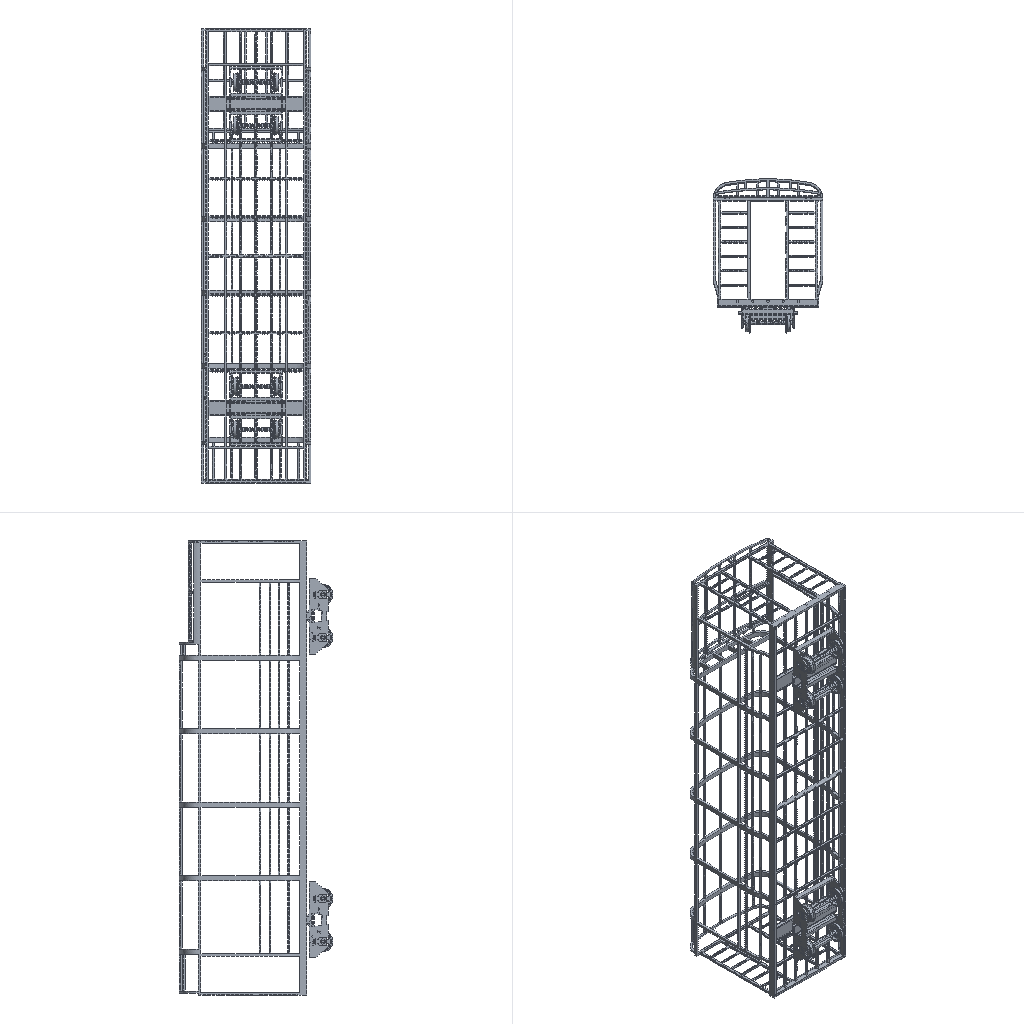Simulation study | ansys workbench
Set-up summary:
category,name,step,type,value,unit,region
solver,ansys_workbench
units,mm-N-s-tonne (MPa),,stated,"/units,MPA"
analysis,LS1,,static
load_step,LS1,LS1,static,nsubst=1; time=1
mesh,nodes,,,844922
mesh,elements,,,484857
element_type,SOLID187,,,440747
element_type,CONTA174,,,29118
element_type,TARGE170,,,10972
element_type,SOLID186,,,4020
material,Structural Steel,,E,200000,tonne s^-2 mm^-1
material,Structural Steel,,nu,0.3
material,Structural Steel,,density,7.85e-09,tonne mm^-3
material,Structural Steel,,conductivity,60.5,tonne mm s^-3 C^-1
material,Structural Steel,,specific_heat,4.34e+08,mm^2 s^-2 C^-1
material,Structural Steel,,cte,1.2e-05,C^-1
material,Structural Steel,,permeability,10000
material,Structural Steel,,resistivity,0.00017,ohm mm
load,,LS1,moment,"2.62e+06 [dir=(1, 0, 0) n=12]",,all
load,,LS1,force,"4284 [dir=(-1, 0, 0) n=3]",,all
load,ACEL,LS1,gravity (ACEL; gravity acts opposite),"9828.46 [dir=(0.02659, -0.9978, 0.06105)]",,all
bc,Constant Zero Displacement X,model,fixed,[dofs=UX],,_DISPZEROUX
bc,Constant Zero Displacement Y,model,fixed,[dofs=UY],,_DISPZEROUY
bc,Constant Zero Displacement Z,model,fixed,[dofs=UZ],,_DISPZEROUZ
contact,Contact Region 10,,bonded (always),element=CONTA174
contact,Contact Region 11,,bonded (always),element=CONTA174
contact,Contact Region 12,,bonded (always),element=CONTA174
contact,Contact Region 13,,bonded (always),element=CONTA174
contact,Contact Region 14,,bonded (always),element=CONTA174
contact,Contact Region 15,,bonded (always),element=CONTA174
contact,Contact Region 16,,bonded (always),element=CONTA174
contact,Contact Region 17,,bonded (always),element=CONTA174
contact,Contact Region 18,,bonded (always),element=CONTA174
contact,Contact Region 19,,bonded (always),element=CONTA174
contact,Contact Region 20,,bonded (always),element=CONTA174
contact,Contact Region 21,,bonded (always),element=CONTA174
contact,Contact Region 22,,bonded (always),element=CONTA174
contact,Contact Region 23,,bonded (always),element=CONTA174
contact,Contact Region 24,,bonded (always),element=CONTA174
contact,Contact Region 25,,bonded (always),element=CONTA174
contact,Contact Region 26,,bonded (always),element=CONTA174
contact,Contact Region 27,,bonded (always),element=CONTA174
contact,Contact Region 28,,bonded (always),element=CONTA174
contact,Contact Region 29,,bonded (always),element=CONTA174
contact,Contact Region 30,,bonded (always),element=CONTA174
contact,Contact Region 31,,bonded (always),element=CONTA174
contact,Contact Region 32,,bonded (always),element=CONTA174
contact,Contact Region 33,,bonded (always),element=CONTA174
contact,Contact Region 34,,bonded (always),element=CONTA174
contact,Contact Region 35,,bonded (always),element=CONTA174
contact,Contact Region 36,,bonded (always),element=CONTA174
contact,Contact Region 37,,bonded (always),element=CONTA174
contact,Contact Region 38,,bonded (always),element=CONTA174
contact,Contact Region 39,,bonded (always),element=CONTA174
contact,Contact Region 40,,bonded (always),element=CONTA174
contact,Contact Region 41,,bonded (always),element=CONTA174
contact,Contact Region 42,,bonded (always),element=CONTA174
contact,Contact Region 43,,bonded (always),element=CONTA174
contact,Contact Region 44,,bonded (always),element=CONTA174
contact,Contact Region 45,,bonded (always),element=CONTA174
contact,Contact Region 46,,bonded (always),element=CONTA174
contact,Contact Region 47,,bonded (always),element=CONTA174
contact,Contact Region 48,,bonded (always),element=CONTA174
contact,Contact Region 49,,bonded (always),element=CONTA174
contact,Contact Region 50,,bonded (always),element=CONTA174
contact,Contact Region 51,,bonded (always),element=CONTA174
contact,Contact Region 52,,bonded (always),element=CONTA174
contact,Contact Region 53,,bonded (always),element=CONTA174
contact,Contact Region 54,,bonded (always),element=CONTA174
contact,Contact Region 55,,bonded (always),element=CONTA174
contact,Contact Region 56,,bonded (always),element=CONTA174
contact,Contact Region 57,,bonded (always),element=CONTA174
contact,Contact Region 58,,bonded (always),element=CONTA174
contact,Contact Region 59,,bonded (always),element=CONTA174
contact,Contact Region 60,,bonded (always),element=CONTA174
contact,Contact Region 61,,bonded (always),element=CONTA174
contact,Contact Region 62,,bonded (always),element=CONTA174
contact,Contact Region 63,,bonded (always),element=CONTA174
contact,Contact Region 64,,bonded (always),element=CONTA174
contact,Contact Region 65,,bonded (always),element=CONTA174
contact,Contact Region 66,,bonded (always),element=CONTA174
contact,Contact Region 67,,bonded (always),element=CONTA174
contact,Contact Region 68,,bonded (always),element=CONTA174
contact,Contact Region 69,,bonded (always),element=CONTA174
contact,Contact Region 70,,bonded (always),element=CONTA174
contact,Contact Region 71,,bonded (always),element=CONTA174
contact,Contact Region 72,,bonded (always),element=CONTA174
contact,Contact Region 73,,bonded (always),element=CONTA174
contact,Contact Region 74,,bonded (always),element=CONTA174
contact,Contact Region 75,,bonded (always),element=CONTA174
contact,Contact Region 76,,bonded (always),element=CONTA174
contact,Contact Region 77,,bonded (always),element=CONTA174
contact,Contact Region 78,,bonded (always),element=CONTA174
contact,Contact Region 79,,bonded (always),element=CONTA174
contact,Contact Region 80,,bonded (always),element=CONTA174
contact,Contact Region 81,,bonded (always),element=CONTA174
contact,Contact Region 82,,bonded (always),element=CONTA174
contact,Contact Region 83,,bonded (always),element=CONTA174
contact,Contact Region 84,,bonded (always),element=CONTA174
contact,Contact Region 85,,bonded (always),element=CONTA174
contact,Contact Region 86,,bonded (always),element=CONTA174
contact,Contact Region 87,,bonded (always),element=CONTA174
contact,Contact Region 88,,bonded (always),element=CONTA174
contact,Contact Region 89,,bonded (always),element=CONTA174
contact,Contact Region 90,,bonded (always),element=CONTA174
contact,Contact Region 91,,bonded (always),element=CONTA174
contact,Contact Region 92,,bonded (always),element=CONTA174
contact,Contact Region 93,,bonded (always),element=CONTA174
contact,Contact Region 94,,bonded (always),element=CONTA174
contact,Contact Region 95,,bonded (always),element=CONTA174
contact,Contact Region 96,,bonded (always),element=CONTA174
contact,Contact Region 97,,bonded (always),element=CONTA174
contact,Contact Region 98,,bonded (always),element=CONTA174
contact,Contact Region 99,,bonded (always),element=CONTA174
contact,Contact Region 100,,bonded (always),element=CONTA174
contact,Contact Region 101,,bonded (always),element=CONTA174
contact,Contact Region 102,,bonded (always),element=CONTA174
contact,Contact Region 103,,bonded (always),element=CONTA174
contact,Contact Region 104,,bonded (always),element=CONTA174
contact,Contact Region 105,,bonded (always),element=CONTA174
contact,Contact Region 106,,bonded (always),element=CONTA174
contact,Contact Region 107,,bonded (always),element=CONTA174
contact,Contact Region 108,,bonded (always),element=CONTA174
contact,Contact Region 109,,bonded (always),element=CONTA174
contact,Contact Region 110,,bonded (always),element=CONTA174
contact,Contact Region 111,,bonded (always),element=CONTA174
contact,Contact Region 112,,bonded (always),element=CONTA174
contact,Contact Region 113,,bonded (always),element=CONTA174
contact,Contact Region 114,,bonded (always),element=CONTA174
contact,Contact Region 115,,bonded (always),element=CONTA174
contact,Contact Region 116,,bonded (always),element=CONTA174
contact,Contact Region 117,,bonded (always),element=CONTA174
contact,Contact Region 118,,bonded (always),element=CONTA174
contact,Contact Region 119,,bonded (always),element=CONTA174
contact,Contact Region 120,,bonded (always),element=CONTA174
contact,contact 112,,bonded (always),element=CONTA174
contact,contact 113,,bonded (always),element=CONTA174
contact,contact 114,,bonded (always),element=CONTA174
contact,contact 115,,bonded (always),element=CONTA174
contact,contact 116,,bonded (always),element=CONTA174
contact,contact 117,,bonded (always),element=CONTA174
contact,contact 118,,bonded (always),element=CONTA174
named_set,_DISPZEROUX,,node,2976
named_set,_DISPZEROUY,,node,2976
named_set,_DISPZEROUZ,,node,1488
Ansys APDL input file, long lists of numbers shortened:
/batch
/config,noeldb,1     ! force off writing results to database
*get,_wallstrt,active,,time,wall
! ANSYS input file written by Workbench version 2021 R1
! File used for geometry attach:
/title,_______--____ 4 (E5)
! ****** Begin Custom Load Command Snippet ******
/COM, ACT Extensions:
/COM,     LSDYNA, 2021.1
/COM,
! ****** End   Custom Load Command Snippet ******
*DIM,_wb_ProjectScratch_dir,string,248
_wb_ProjectScratch_dir(1) = ''
*DIM,_wb_SolverFiles_dir,string,248
_wb_SolverFiles_dir(1) = ''
*DIM,_wb_userfiles_dir,string,248
_wb_userfiles_dir(1) = ''
/com,--- Data in consistent NMM units. See Solving Units in the help system for more information.
/units,MPA
/nopr
/wb,file,start              !  signify a WB generated input file
/prep7
! Turn off shape checking because checks already performed inside WB mesher.
! See help system for more information.
SHPP,OFF,,NOWARN
/nolist
etcon,set             ! allow ANSYS to choose best KEYOP's for 180x elements, resets any applicable keyopt to MAPDL defaults
/com,*********** Nodes for the whole assembly ***********
nblock,3,,929390
(1i9,3e20.9e3)
        1     5.000000000E+02    -2.700000000E+02     8.500000000E+01
! (844899 more lines like these left out)
-1
/com,*********** Nodes for all Remote Points ***********
nblock,3
(1i9,3e20.9e3)
   844901     0.000000000E+00    -4.570000000E+02     1.250000000E+03
! (21 more lines like these left out)
-1
/wb,elem,start            !  set before creation of elements
/com,*********** Elements for Body 1 "____-0|NONE" ***********
et,1,187
eblock,19,solid,,219008
(19i9)
        1        1        1        1        0        0        0        0       10        0   225760   496373   499028   502293   501893   835194   841376   835201   835199
! (438015 more lines like these left out)
-1
/com,*********** Elements for Body 2 "______|NONE" ***********
et,2,186
keyo,2,2,1          ! set full integration on SOLID186
eblock,19,solid,,316
(19i9)
        2        2        2        2        0        0        0        0       20        0      914     6556     6586     6589     6565     6931     6901     6898     6922
! (631 more lines like these left out)
-1
/com,*********** Elements for Body 3 "______|NONE[2]" ***********
et,3,186
keyo,3,2,1          ! set full integration on SOLID186
eblock,19,solid,,316
(19i9)
        3        3        3        3        0        0        0        0       20        0     1663    12147    12177    12180    12156    12522    12492    12489    12513
! (631 more lines like these left out)
-1
/com,*********** Elements for Body 4 "______|NONE[3]" ***********
et,4,186
keyo,4,2,1          ! set full integration on SOLID186
eblock,19,solid,,420
(19i9)
        4        4        4        4        0        0        0        0       20        0     1243     9304     9447     9466     9364     9345     9446     9485     9365
! (839 more lines like these left out)
-1
/com,*********** Elements for Body 5 "______|NONE[4]" ***********
et,5,186
keyo,5,2,1          ! set full integration on SOLID186
eblock,19,solid,,420
(19i9)
        5        5        5        5        0        0        0        0       20        0      481     3579     3722     3741     3639     3620     3721     3760     3640
! (839 more lines like these left out)
-1
! (55 more sections like these left out)
/wb,elem,end               !  done creating elements
/com,*********** Send User Defined Coordinate System(s) ***********
csys,0
toffst,273.15,  ! Temperature offset from absolute zero
/com,*********** Set Reference Temperature ***********
tref,22.
/wb,mat,start              !  starting to send materials
/com,*********** Send Materials ***********
Temperature = 'TEMP' ! Temperature
MP,DENS,1,7.85e-09,	! tonne mm^-3
MP,ALPX,1,1.2e-05,	! C^-1
MP,C,1,434000000,	! mm^2 s^-2 C^-1
MP,KXX,1,60.5,	! tonne mm s^-3 C^-1
MP,RSVX,1,0.00017,	! ohm mm
MP,EX,1,200000,	! tonne s^-2 mm^-1
MP,NUXY,1,0.3,
MP,MURX,1,10000,
Temperature = 'TEMP' ! Temperature
MP,DENS,2,7.85e-09,	! tonne mm^-3
MP,ALPX,2,1.2e-05,	! C^-1
MP,C,2,434000000,	! mm^2 s^-2 C^-1
MP,KXX,2,60.5,	! tonne mm s^-3 C^-1
MP,RSVX,2,0.00017,	! ohm mm
MP,EX,2,200000,	! tonne s^-2 mm^-1
MP,NUXY,2,0.3,
MP,MURX,2,10000,
Temperature = 'TEMP' ! Temperature
MP,DENS,3,7.85e-09,	! tonne mm^-3
MP,ALPX,3,1.2e-05,	! C^-1
MP,C,3,434000000,	! mm^2 s^-2 C^-1
MP,KXX,3,60.5,	! tonne mm s^-3 C^-1
MP,RSVX,3,0.00017,	! ohm mm
MP,EX,3,200000,	! tonne s^-2 mm^-1
MP,NUXY,3,0.3,
MP,MURX,3,10000,
Temperature = 'TEMP' ! Temperature
MP,DENS,4,7.85e-09,	! tonne mm^-3
MP,ALPX,4,1.2e-05,	! C^-1
MP,C,4,434000000,	! mm^2 s^-2 C^-1
MP,KXX,4,60.5,	! tonne mm s^-3 C^-1
MP,RSVX,4,0.00017,	! ohm mm
MP,EX,4,200000,	! tonne s^-2 mm^-1
MP,NUXY,4,0.3,
MP,MURX,4,10000,
Temperature = 'TEMP' ! Temperature
MP,DENS,5,7.85e-09,	! tonne mm^-3
MP,ALPX,5,1.2e-05,	! C^-1
MP,C,5,434000000,	! mm^2 s^-2 C^-1
MP,KXX,5,60.5,	! tonne mm s^-3 C^-1
MP,RSVX,5,0.00017,	! ohm mm
MP,EX,5,200000,	! tonne s^-2 mm^-1
MP,NUXY,5,0.3,
MP,MURX,5,10000,
Temperature = 'TEMP' ! Temperature
MP,DENS,6,7.85e-09,	! tonne mm^-3
MP,ALPX,6,1.2e-05,	! C^-1
MP,C,6,434000000,	! mm^2 s^-2 C^-1
MP,KXX,6,60.5,	! tonne mm s^-3 C^-1
MP,RSVX,6,0.00017,	! ohm mm
MP,EX,6,200000,	! tonne s^-2 mm^-1
MP,NUXY,6,0.3,
MP,MURX,6,10000,
Temperature = 'TEMP' ! Temperature
MP,DENS,7,7.85e-09,	! tonne mm^-3
MP,ALPX,7,1.2e-05,	! C^-1
MP,C,7,434000000,	! mm^2 s^-2 C^-1
MP,KXX,7,60.5,	! tonne mm s^-3 C^-1
MP,RSVX,7,0.00017,	! ohm mm
MP,EX,7,200000,	! tonne s^-2 mm^-1
MP,NUXY,7,0.3,
MP,MURX,7,10000,
Temperature = 'TEMP' ! Temperature
MP,DENS,8,7.85e-09,	! tonne mm^-3
MP,ALPX,8,1.2e-05,	! C^-1
MP,C,8,434000000,	! mm^2 s^-2 C^-1
MP,KXX,8,60.5,	! tonne mm s^-3 C^-1
MP,RSVX,8,0.00017,	! ohm mm
MP,EX,8,200000,	! tonne s^-2 mm^-1
MP,NUXY,8,0.3,
MP,MURX,8,10000,
Temperature = 'TEMP' ! Temperature
MP,DENS,9,7.85e-09,	! tonne mm^-3
MP,ALPX,9,1.2e-05,	! C^-1
MP,C,9,434000000,	! mm^2 s^-2 C^-1
MP,KXX,9,60.5,	! tonne mm s^-3 C^-1
MP,RSVX,9,0.00017,	! ohm mm
MP,EX,9,200000,	! tonne s^-2 mm^-1
! (461 more lines like these left out)
/wb,mat,end                !  done sending materials
!************************* Model Summary ********************
!____-0|NONE,	结构钢,	matid,	1
!______|NONE,	结构钢,	matid,	2
!______|NONE[2],	结构钢,	matid,	3
! (59 more lines like these left out)
*get,_xmin,node,,mnloc,x
*get,_ymin,node,,mnloc,y
*get,_zmin,node,,mnloc,z
*get,_xmax,node,,mxloc,x
*get,_ymax,node,,mxloc,y
*get,_zmax,node,,mxloc,z
_ASMDIAG=(_xmax-_xmin)*(_xmax-_xmin)+(_ymax-_ymin)*(_ymax-_ymin)+(_zmax-_zmin)*(_zmax-_zmin)
_ASMDIAG=SQRT(_ASMDIAG)
/wb,contact,start          !  starting to send contact
/com,*********** Create Contact "接触区域 10" ***********
/com,            Real Constant Set For Above Contact Is 62 & 61
*set,tid,62
*set,cid,61
r,tid
r,cid
et,tid,170
et,cid,174
eblock,10,,,42
(15i9)
   662850       62       62       62        0     6714     6723     6734     6734     7990     8015     6734     7992
! (41 more lines like these left out)
-1
eblock,10,,,42
(15i9)
   662892       61       61       61        0     6714     6723     6734     6734     7990     8015     6734     7992
! (41 more lines like these left out)
-1
eblock,10,,,21
(15i9)
   662934       61       62       61        0     9885    10045     9244     9244    11813    10203     9244    10202
! (20 more lines like these left out)
-1
eblock,10,,,21
(15i9)
   662955       62       61       62        0     9885    10045     9244     9244    11813    10203     9244    10202
! (20 more lines like these left out)
-1
keyo,cid,8,2               ! auto create asymmetric contact (from Program Controlled setting)
keyo,cid,10,0              ! adjust contact stiffness each NR iteration (from Program Controlled setting)
keyo,cid,12,5              ! bonded always
keyo,cid,18,1              ! small sliding turned on by application
keyo,cid,2,0               ! augmented Lagrange (from Program Controlled setting)
keyo,cid,4,0               ! on Gauss point (from Program Controlled setting)
keyo,cid,9,1               ! ignore initial gaps/penetration
keyo,cid,7,0               ! No Prediction
rmod,tid,3,10.      ! FKN
rmod,tid,5,0.       ! ICONT
rmod,tid,6,0.       ! PINB
rmod,tid,10,0.      ! CNOF
rmod,tid,12,0.      ! FKT
rmod,tid,36,14962   ! WB DSID
rmod,cid,3,10.      ! FKN
rmod,cid,5,0.       ! ICONT
rmod,cid,6,0.       ! PINB
rmod,cid,10,0.      ! CNOF
rmod,cid,12,0.      ! FKT
rmod,cid,36,14962   ! WB DSID
/com,*********** Create Contact "接触区域 11" ***********
/com,            Real Constant Set For Above Contact Is 64 & 63
*set,tid,64
*set,cid,63
r,tid
r,cid
et,tid,170
et,cid,174
eblock,10,,,48
(15i9)
   662976       64       64       64        0     6688     6733     6595     6595     7938     7613     6595     7610
! (47 more lines like these left out)
-1
eblock,10,,,48
(15i9)
   663024       63       63       63        0     6688     6733     6595     6595     7938     7613     6595     7610
! (47 more lines like these left out)
-1
eblock,10,,,21
(15i9)
   663072       63       64       63        0     3534     3522     3523     3523     4485     4484     3523     4488
! (20 more lines like these left out)
-1
eblock,10,,,21
(15i9)
   663093       64       63       64        0     3534     3522     3523     3523     4485     4484     3523     4488
! (20 more lines like these left out)
-1
keyo,cid,8,2               ! auto create asymmetric contact (from Program Controlled setting)
keyo,cid,10,0              ! adjust contact stiffness each NR iteration (from Program Controlled setting)
keyo,cid,12,5              ! bonded always
keyo,cid,18,1              ! small sliding turned on by application
keyo,cid,2,0               ! augmented Lagrange (from Program Controlled setting)
keyo,cid,4,0               ! on Gauss point (from Program Controlled setting)
keyo,cid,9,1               ! ignore initial gaps/penetration
keyo,cid,7,0               ! No Prediction
rmod,tid,3,10.      ! FKN
rmod,tid,5,0.       ! ICONT
rmod,tid,6,0.       ! PINB
rmod,tid,10,0.      ! CNOF
rmod,tid,12,0.      ! FKT
rmod,tid,36,14965   ! WB DSID
rmod,cid,3,10.      ! FKN
rmod,cid,5,0.       ! ICONT
rmod,cid,6,0.       ! PINB
rmod,cid,10,0.      ! CNOF
rmod,cid,12,0.      ! FKT
rmod,cid,36,14965   ! WB DSID
/com,*********** Create Contact "接触区域 12" ***********
/com,            Real Constant Set For Above Contact Is 66 & 65
*set,tid,66
*set,cid,65
r,tid
r,cid
et,tid,170
et,cid,174
eblock,10,,,16
(15i9)
   663114       66       66       66        0     6741     6708     6696     6709     7977     7955     7956     7980
! (15 more lines like these left out)
-1
eblock,10,,,16
(15i9)
   663130       65       65       65        0     6741     6708     6696     6709     7977     7955     7956     7980
! (15 more lines like these left out)
-1
eblock,10,,,12
(15i9)
   663146       65       66       65        0     1744     1745     1761     1756     2255     2259     2289     2257
! (11 more lines like these left out)
-1
eblock,10,,,12
(15i9)
   663158       66       65       66        0     1744     1745     1761     1756     2255     2259     2289     2257
! (11 more lines like these left out)
-1
keyo,cid,8,2               ! auto create asymmetric contact (from Program Controlled setting)
keyo,cid,10,0              ! adjust contact stiffness each NR iteration (from Program Controlled setting)
keyo,cid,12,5              ! bonded always
keyo,cid,18,1              ! small sliding turned on by application
keyo,cid,2,0               ! augmented Lagrange (from Program Controlled setting)
keyo,cid,4,0               ! on Gauss point (from Program Controlled setting)
keyo,cid,9,1               ! ignore initial gaps/penetration
keyo,cid,7,0               ! No Prediction
rmod,tid,3,10.      ! FKN
rmod,tid,5,0.       ! ICONT
rmod,tid,6,0.       ! PINB
rmod,tid,10,0.      ! CNOF
rmod,tid,12,0.      ! FKT
rmod,tid,36,14968   ! WB DSID
rmod,cid,3,10.      ! FKN
rmod,cid,5,0.       ! ICONT
rmod,cid,6,0.       ! PINB
rmod,cid,10,0.      ! CNOF
rmod,cid,12,0.      ! FKT
rmod,cid,36,14968   ! WB DSID
/com,*********** Create Contact "接触区域 13" ***********
/com,            Real Constant Set For Above Contact Is 68 & 67
*set,tid,68
*set,cid,67
r,tid
r,cid
et,tid,170
et,cid,174
eblock,10,,,15
(15i9)
   663170       68       68       68        0     6738     6691     6692     6739     7945     7944     7948     8042
! (14 more lines like these left out)
-1
eblock,10,,,15
(15i9)
   663185       67       67       67        0     6738     6691     6692     6739     7945     7944     7948     8042
! (14 more lines like these left out)
-1
eblock,10,,,12
(15i9)
   663200       67       68       67        0       21       16        4        5      549      517      515      519
! (11 more lines like these left out)
-1
eblock,10,,,12
(15i9)
   663212       68       67       68        0       21       16        4        5      549      517      515      519
! (11 more lines like these left out)
-1
keyo,cid,8,2               ! auto create asymmetric contact (from Program Controlled setting)
keyo,cid,10,0              ! adjust contact stiffness each NR iteration (from Program Controlled setting)
keyo,cid,12,5              ! bonded always
keyo,cid,18,1              ! small sliding turned on by application
keyo,cid,2,0               ! augmented Lagrange (from Program Controlled setting)
keyo,cid,4,0               ! on Gauss point (from Program Controlled setting)
keyo,cid,9,1               ! ignore initial gaps/penetration
keyo,cid,7,0               ! No Prediction
rmod,tid,3,10.      ! FKN
rmod,tid,5,0.       ! ICONT
rmod,tid,6,0.       ! PINB
rmod,tid,10,0.      ! CNOF
rmod,tid,12,0.      ! FKT
rmod,tid,36,14971   ! WB DSID
rmod,cid,3,10.      ! FKN
rmod,cid,5,0.       ! ICONT
rmod,cid,6,0.       ! PINB
rmod,cid,10,0.      ! CNOF
rmod,cid,12,0.      ! FKT
rmod,cid,36,14971   ! WB DSID
/com,*********** Create Contact "接触区域 14" ***********
/com,            Real Constant Set For Above Contact Is 70 & 69
*set,tid,70
*set,cid,69
r,tid
r,cid
et,tid,170
et,cid,174
eblock,10,,,33
(15i9)
   663224       70       70       70        0     7129     7127     7128     7133     8908     8907     8909     8911
! (32 more lines like these left out)
-1
eblock,10,,,33
(15i9)
   663257       69       69       69        0     7129     7127     7128     7133     8908     8907     8909     8911
! (32 more lines like these left out)
-1
eblock,10,,,170
(15i9)
   663290       69       70       69        0    17468    17488    17473    17473    26290    26306    17473    26287
! (169 more lines like these left out)
-1
eblock,10,,,170
(15i9)
   663460       70       69       70        0    17468    17488    17473    17473    26290    26306    17473    26287
! (169 more lines like these left out)
-1
keyo,cid,8,2               ! auto create asymmetric contact (from Program Controlled setting)
keyo,cid,10,0              ! adjust contact stiffness each NR iteration (from Program Controlled setting)
keyo,cid,12,5              ! bonded always
keyo,cid,18,1              ! small sliding turned on by application
keyo,cid,2,0               ! augmented Lagrange (from Program Controlled setting)
keyo,cid,4,0               ! on Gauss point (from Program Controlled setting)
keyo,cid,9,1               ! ignore initial gaps/penetration
keyo,cid,7,0               ! No Prediction
rmod,tid,3,10.      ! FKN
rmod,tid,5,0.       ! ICONT
rmod,tid,6,0.       ! PINB
rmod,tid,10,0.      ! CNOF
rmod,tid,12,0.      ! FKT
rmod,tid,36,14974   ! WB DSID
rmod,cid,3,10.      ! FKN
rmod,cid,5,0.       ! ICONT
rmod,cid,6,0.       ! PINB
rmod,cid,10,0.      ! CNOF
rmod,cid,12,0.      ! FKT
rmod,cid,36,14974   ! WB DSID
! (106 more sections like these left out)
/wb,contact,end            !  done creating contacts
/golist
/wb,load,start             !  starting to send loads
/com,******* Constant Zero Displacement X *******
CMBLOCK,_DISPZEROUX,NODE,     2976
(8i10)
     33525     33526     33527     33528     33529     33530     33531     33532
! (371 more lines like these left out)
cmsel,s,_DISPZEROUX
d,all,ux,0
nsel,all
/com,******* Constant Zero Displacement Y *******
CMBLOCK,_DISPZEROUY,NODE,     2976
(8i10)
     33525     33526     33527     33528     33529     33530     33531     33532
! (371 more lines like these left out)
cmsel,s,_DISPZEROUY
d,all,uy,0
nsel,all
/com,******* Constant Zero Displacement Z *******
CMBLOCK,_DISPZEROUZ,NODE,     1488
(8i10)
     33525     33526     33527     33528     33529     33530     33531     33532
! (185 more lines like these left out)
cmsel,s,_DISPZEROUZ
d,all,uz,0
nsel,all
/com,*********** Create Remote Point "内部远程点" ***********
! -------- Remote Point Used by "力矩" --------
*set,tid,284
*set,cid,283
et,cid,174
et,tid,170
keyo,tid,2,1               ! Don't fix the pilot node
keyo,tid,4,0               ! Activate all DOF's due to large deformation
keyo,cid,12,5              ! Bonded Contact
keyo,cid,4,1               ! Deformable RBE3 style load
keyo,cid,2,2               ! MPC style contact
eblock,10,,,358
(15i9)
   684794      283      283      283        0    38713    38614    38728    38728    39254    39255    38728    40038
! (357 more lines like these left out)
-1
*set,_npilot,844913
_npilot15445=_npilot
type,tid
mat ,cid
real,cid
tshape,pilo
en,685152,_npilot
tshape
/com,*********** Create Remote Point "内部远程点 2" ***********
! -------- Remote Point Used by "力矩 2" --------
*set,tid,286
*set,cid,285
et,cid,174
et,tid,170
keyo,tid,2,1               ! Don't fix the pilot node
keyo,tid,4,0               ! Activate all DOF's due to large deformation
keyo,cid,12,5              ! Bonded Contact
keyo,cid,4,1               ! Deformable RBE3 style load
keyo,cid,2,2               ! MPC style contact
eblock,10,,,360
(15i9)
   685153      285      285      285        0    71272    71189    71399    71399    72063    72066    71399    72735
! (359 more lines like these left out)
-1
*set,_npilot,844914
_npilot15448=_npilot
type,tid
mat ,cid
real,cid
tshape,pilo
en,685513,_npilot
tshape
/com,*********** Create Remote Point "内部远程点 3" ***********
! -------- Remote Point Used by "力矩 3" --------
*set,tid,288
*set,cid,287
et,cid,174
et,tid,170
keyo,tid,2,1               ! Don't fix the pilot node
keyo,tid,4,0               ! Activate all DOF's due to large deformation
keyo,cid,12,5              ! Bonded Contact
keyo,cid,4,1               ! Deformable RBE3 style load
keyo,cid,2,2               ! MPC style contact
eblock,10,,,358
(15i9)
   685514      287      287      287        0    27853    27754    27868    27868    28394    28395    27868    29178
! (357 more lines like these left out)
-1
*set,_npilot,844915
_npilot15451=_npilot
type,tid
mat ,cid
real,cid
tshape,pilo
en,685872,_npilot
tshape
/com,*********** Create Remote Point "内部远程点 4" ***********
! -------- Remote Point Used by "力矩 4" --------
*set,tid,290
*set,cid,289
et,cid,174
et,tid,170
keyo,tid,2,1               ! Don't fix the pilot node
keyo,tid,4,0               ! Activate all DOF's due to large deformation
keyo,cid,12,5              ! Bonded Contact
keyo,cid,4,1               ! Deformable RBE3 style load
keyo,cid,2,2               ! MPC style contact
eblock,10,,,360
(15i9)
   685873      289      289      289        0    60036    59953    60163    60163    60827    60830    60163    61499
! (359 more lines like these left out)
-1
*set,_npilot,844916
_npilot15454=_npilot
type,tid
mat ,cid
real,cid
tshape,pilo
en,686233,_npilot
tshape
/com,*********** Create Remote Point "内部远程点 17" ***********
! -------- Remote Point Used by "乘客重量" --------
*set,tid,292
*set,cid,291
et,cid,174
et,tid,170
keyo,tid,2,1               ! Don't fix the pilot node
keyo,tid,4,0               ! Activate all DOF's due to large deformation
keyo,cid,12,5              ! Bonded Contact
keyo,cid,4,1               ! Deformable RBE3 style load
keyo,cid,2,2               ! MPC style contact
eblock,10,,,6072
(15i9)
   686234      291      291      291        0   148608   149004   149355   149355   346755   349666   149355   346758
! (6071 more lines like these left out)
-1
*set,_npilot,844917
_npilot15533=_npilot
type,tid
mat ,cid
real,cid
tshape,pilo
en,692306,_npilot
tshape
! (2 more sections like these left out)
/com,*********** Construct Moment Using Remote Attachment ***********
/com,*********** Construct Moment Using Remote Attachment ***********
*DIM,_loadvari15447x,TABLE,2,1,1,TIME,
! Time values
_loadvari15447x(1,0,1) = 0.
_loadvari15447x(2,0,1) = 1.
! Load values
_loadvari15447x(1,1,1) = 0.
_loadvari15447x(2,1,1) = 655000.
*DIM,_loadvari15447y,TABLE,2,1,1,TIME,
! Time values
_loadvari15447y(1,0,1) = 0.
_loadvari15447y(2,0,1) = 1.
! Load values
_loadvari15447y(1,1,1) = 0.
_loadvari15447y(2,1,1) = 0.
*DIM,_loadvari15447z,TABLE,2,1,1,TIME,
! Time values
_loadvari15447z(1,0,1) = 0.
_loadvari15447z(2,0,1) = 1.
! Load values
_loadvari15447z(1,1,1) = 0.
_loadvari15447z(2,1,1) = 0.
/com,*********** Construct Moment Using Remote Attachment ***********
*DIM,_loadvari15450x,TABLE,2,1,1,TIME,
! Time values
_loadvari15450x(1,0,1) = 0.
_loadvari15450x(2,0,1) = 1.
! Load values
_loadvari15450x(1,1,1) = 0.
_loadvari15450x(2,1,1) = 655000.
*DIM,_loadvari15450y,TABLE,2,1,1,TIME,
! Time values
_loadvari15450y(1,0,1) = 0.
_loadvari15450y(2,0,1) = 1.
! Load values
_loadvari15450y(1,1,1) = 0.
_loadvari15450y(2,1,1) = 0.
*DIM,_loadvari15450z,TABLE,2,1,1,TIME,
! Time values
_loadvari15450z(1,0,1) = 0.
_loadvari15450z(2,0,1) = 1.
! Load values
_loadvari15450z(1,1,1) = 0.
_loadvari15450z(2,1,1) = 0.
/com,*********** Construct Moment Using Remote Attachment ***********
*DIM,_loadvari15453x,TABLE,2,1,1,TIME,
! Time values
_loadvari15453x(1,0,1) = 0.
_loadvari15453x(2,0,1) = 1.
! Load values
_loadvari15453x(1,1,1) = 0.
_loadvari15453x(2,1,1) = 655000.
*DIM,_loadvari15453y,TABLE,2,1,1,TIME,
! Time values
_loadvari15453y(1,0,1) = 0.
_loadvari15453y(2,0,1) = 1.
! Load values
_loadvari15453y(1,1,1) = 0.
_loadvari15453y(2,1,1) = 0.
*DIM,_loadvari15453z,TABLE,2,1,1,TIME,
! Time values
_loadvari15453z(1,0,1) = 0.
_loadvari15453z(2,0,1) = 1.
! Load values
_loadvari15453z(1,1,1) = 0.
_loadvari15453z(2,1,1) = 0.
/com,*********** Construct Remote Force ***********
*DIM,_loadvari15642x,TABLE,2,1,1,TIME,
! Time values
_loadvari15642x(1,0,1) = 0.
_loadvari15642x(2,0,1) = 1.
! Load values
_loadvari15642x(1,1,1) = 0.
_loadvari15642x(2,1,1) = -4284.
*DIM,_loadvari15642y,TABLE,2,1,1,TIME,
! Time values
_loadvari15642y(1,0,1) = 0.
_loadvari15642y(2,0,1) = 1.
! Load values
_loadvari15642y(1,1,1) = 0.
_loadvari15642y(2,1,1) = 0.
*DIM,_loadvari15642z,TABLE,2,1,1,TIME,
! Time values
_loadvari15642z(1,0,1) = 0.
_loadvari15642z(2,0,1) = 1.
! Load values
_loadvari15642z(1,1,1) = 0.
_loadvari15642z(2,1,1) = 0.
/com,*********** Construct Remote Mass Using Remote Attachment ***********
*set,_tid,297
et,_tid,21           ! MASS21 element
type,_tid
mat ,_tid
real,_tid
keyo,_tid,3,2        ! 3d mass without rotary inertia
r,_tid,2.8
en,702947,844917
/com,*********** Construct Remote Mass Using Remote Attachment ***********
*set,_tid,298
et,_tid,21           ! MASS21 element
type,_tid
mat ,_tid
real,_tid
keyo,_tid,3,2        ! 3d mass without rotary inertia
r,_tid,0.45
en,702948,844918
/gst,on,on
fini
*get,_numnode,node,0,count
*get,_numelem,elem,0,count
*get, _MAXELEMNUM, elem, 0, NUM, MAX
*get, _MAXNODENUM, node, 0, NUM, MAX
*get, _MAXELEMTYPE, etyp, 0, NUM, MAX
*get, _MAXREALCONST, real, 0, NUM, MAX
/go
/wb,load,end               !  done creating loads
/com,--- Number of total nodes = %_numnode%
/com,--- Number of contact elements = 40090
/com,--- Number of spring elements = 0
/com,--- Number of bearing elements = 0
/com,--- Number of solid elements = 444767
/com,--- Number of condensed parts = 0
/com,--- Number of total elements = %_numelem%
*get,_wallbsol,active,,time,wall
/com,****************************************************************************
/com,*************************    SOLUTION       ********************************
/com,****************************************************************************
/solu
antype,0                   ! static analysis
nlgeom,on                  ! Turn on Large Deformation Effects
_thickRatio=0.1     ! Ratio of thick parts in the model
eqsl,sparse,,,,,1
cntr,print,1               ! print out contact info and also make no initial contact an error
cntr,out,yes               ! write contact output to file.cmn due to many contact pairs present
dmpoption,emat,no             ! Don't combine emat file for DANSYS
dmpoption,esav,no             ! Don't combine esav file for DANSYS
nldiag,cont,iter           ! print out contact info each equilibrium iteration
rescontrol,define,last,last,,dele	   ! Program Controlled
/com,****************************************************
/com,******************* SOLVE FOR LS 1 OF 1 ****************
nsel,s,node,,844913
f,all,mx,655000.
f,all,my,0.
f,all,mz,0.
nsel,s,node,,844914
f,all,mx,%_loadvari15447x%
f,all,my,%_loadvari15447y%
f,all,mz,%_loadvari15447z%
nsel,s,node,,844915
f,all,mx,%_loadvari15450x%
f,all,my,%_loadvari15450y%
f,all,mz,%_loadvari15450z%
nsel,s,node,,844916
f,all,mx,%_loadvari15453x%
f,all,my,%_loadvari15453y%
f,all,mz,%_loadvari15453z%
nsel,all
nsel,s,node,,844922
f,all,fx,%_loadvari15642x%
f,all,fy,%_loadvari15642y%
f,all,fz,%_loadvari15642z%
nsel,all
acel,-261.3,9806.65,-600.
/nopr
/gopr
/nolist
autots,on                  ! Workbench Program Controlled automatic time stepping
nsub,1,10,1                ! due to presence of general nonlinear
time,1.
outres,erase
outres,all,none
outres,nsol,all,
outres,rsol,all
outres,eangl,all
outres,etmp,all
outres,veng,all
outres,strs,all,
outres,epel,all,
outres,eppl,all,
outres,cont,all,
! *********** WB SOLVE COMMAND ***********
! check interactive state
*get,ANSINTER_,active,,int
*if,ANSINTER_,ne,0,then
/eof
*endif
solve
/com *************** Write FE CONNECTORS *********
CEWRITE,file,ce,,INTE
/com,****************************************************
/com,*************** FINISHED SOLVE FOR LS 1 *************
*get,_wallasol,active,,time,wall
/nopr
*get,_numnode,node,0,count
*get,_numelem,elem,0,count
*get, _MAXELEMNUM, elem, 0, NUM, MAX
*get, _MAXNODENUM, node, 0, NUM, MAX,,,INTERNAL
*get, _MAXELEMTYPE, etyp, 0, NUM, MAX
*get, _MAXREALCONST, real, 0, NUM, MAX
/gopr
/post1
xmlo,ENCODING,ISO-8859-1
xmlo,parm
/xml,parm,xml
fini
/gopr
*get,_walldone,active,,time,wall
_preptime=(_wallbsol-_wallstrt)*3600
_solvtime=(_wallasol-_wallbsol)*3600
_posttime=(_walldone-_wallasol)*3600
_totaltim=(_walldone-_wallstrt)*3600
*get,_dlbratio,active,0,solu,dlbr
*get,_combtime,active,0,solu,comb
/com,--- Total number of nodes = %_numnode%
/com,--- Total number of elements = %_numelem%
/com,--- Element load balance ratio = %_dlbratio%
/com,--- Time to combine distributed files = %_combtime%
/wb,file,end               ! done with WB generated input
Results summary:
result,analyses[0].index,,,1
result,analyses[0].system,,,SYS-4
result,analyses[0].deck,,,deck.dat
result,analyses[0].solve_status,,,completed
result,analyses[0].analysis_type,,,static
result,analyses[0].physics,,,mechanical
result,analyses[0].unit_system,,,"NMM: mm, ton, N, s, mV, mA, degC"
result,analyses[0].n_sets,,,1
result,analyses[0].load_steps[0].set,set=1,,1
result,analyses[0].load_steps[0].time_or_freq,set=1,,1
result,analyses[0].load_steps[0].max_displacement_magnitude,set=1,,4.066
result,analyses[0].load_steps[0].max_von_mises_nodal,set=1,,139.109
result,analyses[0].load_steps[0].reaction_force_sum_xyz[1],set=1,,1716.05
result,analyses[0].load_steps[0].reaction_force_sum_xyz[2],set=1,,96375.6
result,analyses[0].load_steps[0].reaction_force_sum_xyz[3],set=1,,-5896.55
result,geometry_export[0][0],,,.step
result,geometry_export[0][1],,,ok
result,geometry_export[0][2],,,329